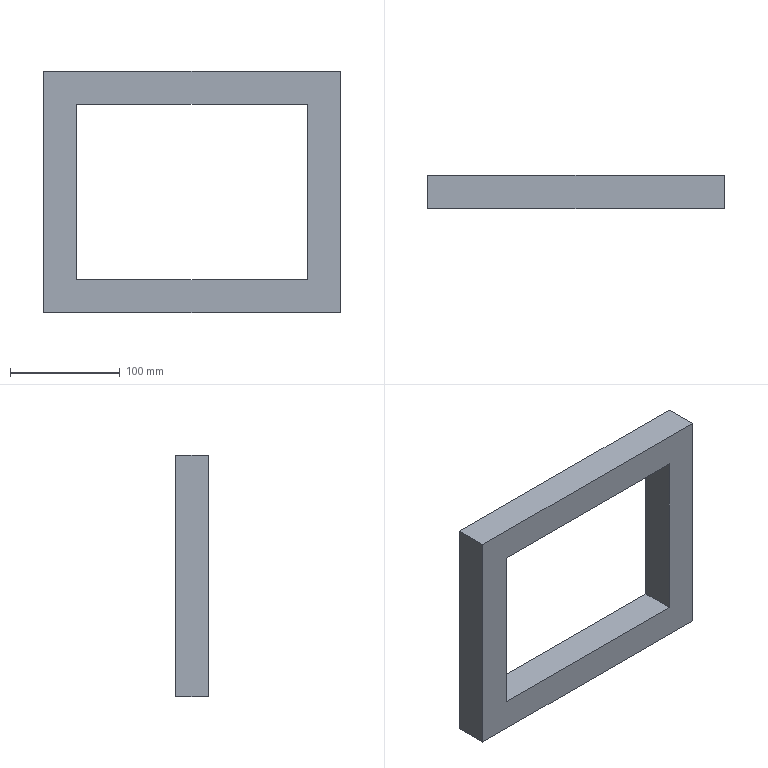Part | SolidWorks | features Extrusion 1, HoleWzd 1 | 1 solid | 58 faces | box 270 x 30 x 220 mm | volume 767460 mm3 | cone 32 | cylinder 16 | plane 10 | commonest cylinder face diameters 6.8 x16
STEP:
#1=CARTESIAN_POINT('',(0.,29.375,-98.4));
#2=VERTEX_POINT('',#1);
#3=CARTESIAN_POINT('',(0.,29.375,-91.6));
#4=VERTEX_POINT('',#3);
#5=CARTESIAN_POINT('',(0.,29.375,-95.));
#6=DIRECTION('',(0.,1.,0.));
#7=DIRECTION('',(0.,0.,1.));
#8=AXIS2_PLACEMENT_3D('',#5,#6,#7);
#9=CIRCLE('',#8,3.4);
#10=EDGE_CURVE('',#2,#4,#9,.T.);
#11=ORIENTED_EDGE('',*,*,#10,.F.);
#12=CARTESIAN_POINT('',(0.,30.,-99.025));
#13=VERTEX_POINT('',#12);
#14=CARTESIAN_POINT('',(0.,30.,-99.025));
#15=DIRECTION('',(0.,0.7071,-0.7071));
#16=VECTOR('',#15,1000.);
#17=LINE('',#14,#16);
#18=EDGE_CURVE('',#2,#13,#17,.T.);
#19=ORIENTED_EDGE('',*,*,#18,.T.);
#20=CARTESIAN_POINT('',(0.,30.,-90.975));
#21=VERTEX_POINT('',#20);
#22=CARTESIAN_POINT('',(0.,30.,-95.));
#23=DIRECTION('',(0.,1.,0.));
#24=DIRECTION('',(0.,0.,1.));
#25=AXIS2_PLACEMENT_3D('',#22,#23,#24);
#26=CIRCLE('',#25,4.025);
#27=EDGE_CURVE('',#13,#21,#26,.T.);
#28=ORIENTED_EDGE('',*,*,#27,.T.);
#29=CARTESIAN_POINT('',(0.,30.,-90.975));
#30=DIRECTION('',(0.,0.7071,0.7071));
#31=VECTOR('',#30,1000.);
#32=LINE('',#29,#31);
#33=EDGE_CURVE('',#4,#21,#32,.T.);
#34=ORIENTED_EDGE('',*,*,#33,.F.);
#35=EDGE_LOOP('',(#11,#19,#28,#34));
#36=FACE_OUTER_BOUND('',#35,.T.);
#37=CARTESIAN_POINT('',(0.,30.,-95.));
#38=DIRECTION('',(0.,1.,0.));
#39=DIRECTION('',(0.,0.,1.));
#40=AXIS2_PLACEMENT_3D('',#37,#38,#39);
#41=CONICAL_SURFACE('',#40,4.025,0.7854);
#42=ADVANCED_FACE('',(#36),#41,.F.);
#43=CARTESIAN_POINT('',(0.,8.293,-98.4));
#44=VERTEX_POINT('',#43);
#45=CARTESIAN_POINT('',(0.,8.293,-91.6));
#46=VERTEX_POINT('',#45);
#47=CARTESIAN_POINT('',(0.,8.293,-95.));
#48=DIRECTION('',(0.,1.,0.));
#49=DIRECTION('',(0.,0.,1.));
#50=AXIS2_PLACEMENT_3D('',#47,#48,#49);
#51=CIRCLE('',#50,3.4);
#52=EDGE_CURVE('',#44,#46,#51,.T.);
#53=ORIENTED_EDGE('',*,*,#52,.F.);
#54=CARTESIAN_POINT('',(0.,30.,-98.4));
#55=DIRECTION('',(0.,1.,0.));
#56=VECTOR('',#55,1000.);
#57=LINE('',#54,#56);
#58=EDGE_CURVE('',#44,#2,#57,.T.);
#59=ORIENTED_EDGE('',*,*,#58,.T.);
#60=ORIENTED_EDGE('',*,*,#10,.T.);
#61=CARTESIAN_POINT('',(0.,30.,-91.6));
#62=DIRECTION('',(0.,1.,0.));
#63=VECTOR('',#62,1000.);
#64=LINE('',#61,#63);
#65=EDGE_CURVE('',#46,#4,#64,.T.);
#66=ORIENTED_EDGE('',*,*,#65,.F.);
#67=EDGE_LOOP('',(#53,#59,#60,#66));
#68=FACE_OUTER_BOUND('',#67,.T.);
#69=CARTESIAN_POINT('',(0.,30.,-95.));
#70=DIRECTION('',(0.,1.,0.));
#71=DIRECTION('',(0.,0.,1.));
#72=AXIS2_PLACEMENT_3D('',#69,#70,#71);
#73=CYLINDRICAL_SURFACE('',#72,3.4);
#74=ADVANCED_FACE('',(#68),#73,.F.);
#75=CARTESIAN_POINT('',(0.,6.25,-95.));
#76=VERTEX_POINT('',#75);
#77=CARTESIAN_POINT('',(0.,8.293,-91.6));
#78=DIRECTION('',(0.,0.515,0.8572));
#79=VECTOR('',#78,1000.);
#80=LINE('',#77,#79);
#81=EDGE_CURVE('',#76,#46,#80,.T.);
#82=ORIENTED_EDGE('',*,*,#81,.F.);
#83=CARTESIAN_POINT('',(0.,8.293,-98.4));
#84=DIRECTION('',(0.,0.515,-0.8572));
#85=VECTOR('',#84,1000.);
#86=LINE('',#83,#85);
#87=EDGE_CURVE('',#76,#44,#86,.T.);
#88=ORIENTED_EDGE('',*,*,#87,.T.);
#89=ORIENTED_EDGE('',*,*,#52,.T.);
#90=EDGE_LOOP('',(#82,#88,#89));
#91=FACE_OUTER_BOUND('',#90,.T.);
#92=CARTESIAN_POINT('',(0.,8.293,-95.));
#93=DIRECTION('',(0.,1.,0.));
#94=DIRECTION('',(0.,0.,1.));
#95=AXIS2_PLACEMENT_3D('',#92,#93,#94);
#96=CONICAL_SURFACE('',#95,3.4,1.03);
#97=ADVANCED_FACE('',(#91),#96,.F.);
#98=CARTESIAN_POINT('',(-120.,29.375,-98.4));
#99=VERTEX_POINT('',#98);
#100=CARTESIAN_POINT('',(-120.,29.375,-91.6));
#101=VERTEX_POINT('',#100);
#102=CARTESIAN_POINT('',(-120.,29.375,-95.));
#103=DIRECTION('',(0.,1.,0.));
#104=DIRECTION('',(0.,0.,1.));
#105=AXIS2_PLACEMENT_3D('',#102,#103,#104);
#106=CIRCLE('',#105,3.4);
#107=EDGE_CURVE('',#99,#101,#106,.T.);
#108=ORIENTED_EDGE('',*,*,#107,.F.);
#109=CARTESIAN_POINT('',(-120.,30.,-99.025));
#110=VERTEX_POINT('',#109);
#111=CARTESIAN_POINT('',(-120.,30.,-99.025));
#112=DIRECTION('',(0.,0.7071,-0.7071));
#113=VECTOR('',#112,1000.);
#114=LINE('',#111,#113);
#115=EDGE_CURVE('',#99,#110,#114,.T.);
#116=ORIENTED_EDGE('',*,*,#115,.T.);
#117=CARTESIAN_POINT('',(-120.,30.,-90.975));
#118=VERTEX_POINT('',#117);
#119=CARTESIAN_POINT('',(-120.,30.,-95.));
#120=DIRECTION('',(0.,1.,0.));
#121=DIRECTION('',(0.,0.,1.));
#122=AXIS2_PLACEMENT_3D('',#119,#120,#121);
#123=CIRCLE('',#122,4.025);
#124=EDGE_CURVE('',#110,#118,#123,.T.);
#125=ORIENTED_EDGE('',*,*,#124,.T.);
#126=CARTESIAN_POINT('',(-120.,30.,-90.975));
#127=DIRECTION('',(0.,0.7071,0.7071));
#128=VECTOR('',#127,1000.);
#129=LINE('',#126,#128);
#130=EDGE_CURVE('',#101,#118,#129,.T.);
#131=ORIENTED_EDGE('',*,*,#130,.F.);
#132=EDGE_LOOP('',(#108,#116,#125,#131));
#133=FACE_OUTER_BOUND('',#132,.T.);
#134=CARTESIAN_POINT('',(-120.,30.,-95.));
#135=DIRECTION('',(0.,1.,0.));
#136=DIRECTION('',(0.,0.,1.));
#137=AXIS2_PLACEMENT_3D('',#134,#135,#136);
#138=CONICAL_SURFACE('',#137,4.025,0.7854);
#139=ADVANCED_FACE('',(#133),#138,.F.);
#140=CARTESIAN_POINT('',(-120.,8.293,-98.4));
#141=VERTEX_POINT('',#140);
#142=CARTESIAN_POINT('',(-120.,8.293,-91.6));
#143=VERTEX_POINT('',#142);
#144=CARTESIAN_POINT('',(-120.,8.293,-95.));
#145=DIRECTION('',(0.,1.,0.));
#146=DIRECTION('',(0.,0.,1.));
#147=AXIS2_PLACEMENT_3D('',#144,#145,#146);
#148=CIRCLE('',#147,3.4);
#149=EDGE_CURVE('',#141,#143,#148,.T.);
#150=ORIENTED_EDGE('',*,*,#149,.F.);
#151=CARTESIAN_POINT('',(-120.,30.,-98.4));
#152=DIRECTION('',(0.,1.,0.));
#153=VECTOR('',#152,1000.);
#154=LINE('',#151,#153);
#155=EDGE_CURVE('',#141,#99,#154,.T.);
#156=ORIENTED_EDGE('',*,*,#155,.T.);
#157=ORIENTED_EDGE('',*,*,#107,.T.);
#158=CARTESIAN_POINT('',(-120.,30.,-91.6));
#159=DIRECTION('',(0.,1.,0.));
#160=VECTOR('',#159,1000.);
#161=LINE('',#158,#160);
#162=EDGE_CURVE('',#143,#101,#161,.T.);
#163=ORIENTED_EDGE('',*,*,#162,.F.);
#164=EDGE_LOOP('',(#150,#156,#157,#163));
#165=FACE_OUTER_BOUND('',#164,.T.);
#166=CARTESIAN_POINT('',(-120.,30.,-95.));
#167=DIRECTION('',(0.,1.,0.));
#168=DIRECTION('',(0.,0.,1.));
#169=AXIS2_PLACEMENT_3D('',#166,#167,#168);
#170=CYLINDRICAL_SURFACE('',#169,3.4);
#171=ADVANCED_FACE('',(#165),#170,.F.);
#172=CARTESIAN_POINT('',(-120.,6.25,-95.));
#173=VERTEX_POINT('',#172);
#174=CARTESIAN_POINT('',(-120.,8.293,-91.6));
#175=DIRECTION('',(0.,0.515,0.8572));
#176=VECTOR('',#175,1000.);
#177=LINE('',#174,#176);
#178=EDGE_CURVE('',#173,#143,#177,.T.);
#179=ORIENTED_EDGE('',*,*,#178,.F.);
#180=CARTESIAN_POINT('',(-120.,8.293,-98.4));
#181=DIRECTION('',(0.,0.515,-0.8572));
#182=VECTOR('',#181,1000.);
#183=LINE('',#180,#182);
#184=EDGE_CURVE('',#173,#141,#183,.T.);
#185=ORIENTED_EDGE('',*,*,#184,.T.);
#186=ORIENTED_EDGE('',*,*,#149,.T.);
#187=EDGE_LOOP('',(#179,#185,#186));
#188=FACE_OUTER_BOUND('',#187,.T.);
#189=CARTESIAN_POINT('',(-120.,8.293,-95.));
#190=DIRECTION('',(0.,1.,0.));
#191=DIRECTION('',(0.,0.,1.));
#192=AXIS2_PLACEMENT_3D('',#189,#190,#191);
#193=CONICAL_SURFACE('',#192,3.4,1.03);
#194=ADVANCED_FACE('',(#188),#193,.F.);
#195=CARTESIAN_POINT('',(-120.,29.375,-3.4));
#196=VERTEX_POINT('',#195);
#197=CARTESIAN_POINT('',(-120.,29.375,3.4));
#198=VERTEX_POINT('',#197);
#199=CARTESIAN_POINT('',(-120.,29.375,0.));
#200=DIRECTION('',(0.,1.,0.));
#201=DIRECTION('',(0.,0.,1.));
#202=AXIS2_PLACEMENT_3D('',#199,#200,#201);
#203=CIRCLE('',#202,3.4);
#204=EDGE_CURVE('',#196,#198,#203,.T.);
#205=ORIENTED_EDGE('',*,*,#204,.F.);
#206=CARTESIAN_POINT('',(-120.,30.,-4.025));
#207=VERTEX_POINT('',#206);
#208=CARTESIAN_POINT('',(-120.,30.,-4.025));
#209=DIRECTION('',(0.,0.7071,-0.7071));
#210=VECTOR('',#209,1000.);
#211=LINE('',#208,#210);
#212=EDGE_CURVE('',#196,#207,#211,.T.);
#213=ORIENTED_EDGE('',*,*,#212,.T.);
#214=CARTESIAN_POINT('',(-120.,30.,4.025));
#215=VERTEX_POINT('',#214);
#216=CARTESIAN_POINT('',(-120.,30.,0.));
#217=DIRECTION('',(0.,1.,0.));
#218=DIRECTION('',(0.,0.,1.));
#219=AXIS2_PLACEMENT_3D('',#216,#217,#218);
#220=CIRCLE('',#219,4.025);
#221=EDGE_CURVE('',#207,#215,#220,.T.);
#222=ORIENTED_EDGE('',*,*,#221,.T.);
#223=CARTESIAN_POINT('',(-120.,30.,4.025));
#224=DIRECTION('',(0.,0.7071,0.7071));
#225=VECTOR('',#224,1000.);
#226=LINE('',#223,#225);
#227=EDGE_CURVE('',#198,#215,#226,.T.);
#228=ORIENTED_EDGE('',*,*,#227,.F.);
#229=EDGE_LOOP('',(#205,#213,#222,#228));
#230=FACE_OUTER_BOUND('',#229,.T.);
#231=CARTESIAN_POINT('',(-120.,30.,0.));
#232=DIRECTION('',(0.,1.,0.));
#233=DIRECTION('',(0.,0.,1.));
#234=AXIS2_PLACEMENT_3D('',#231,#232,#233);
#235=CONICAL_SURFACE('',#234,4.025,0.7854);
#236=ADVANCED_FACE('',(#230),#235,.F.);
#237=CARTESIAN_POINT('',(-120.,8.293,-3.4));
#238=VERTEX_POINT('',#237);
#239=CARTESIAN_POINT('',(-120.,8.293,3.4));
#240=VERTEX_POINT('',#239);
#241=CARTESIAN_POINT('',(-120.,8.293,0.));
#242=DIRECTION('',(0.,1.,0.));
#243=DIRECTION('',(0.,0.,1.));
#244=AXIS2_PLACEMENT_3D('',#241,#242,#243);
#245=CIRCLE('',#244,3.4);
#246=EDGE_CURVE('',#238,#240,#245,.T.);
#247=ORIENTED_EDGE('',*,*,#246,.F.);
#248=CARTESIAN_POINT('',(-120.,30.,-3.4));
#249=DIRECTION('',(0.,1.,0.));
#250=VECTOR('',#249,1000.);
#251=LINE('',#248,#250);
#252=EDGE_CURVE('',#238,#196,#251,.T.);
#253=ORIENTED_EDGE('',*,*,#252,.T.);
#254=ORIENTED_EDGE('',*,*,#204,.T.);
#255=CARTESIAN_POINT('',(-120.,30.,3.4));
#256=DIRECTION('',(0.,1.,0.));
#257=VECTOR('',#256,1000.);
#258=LINE('',#255,#257);
#259=EDGE_CURVE('',#240,#198,#258,.T.);
#260=ORIENTED_EDGE('',*,*,#259,.F.);
#261=EDGE_LOOP('',(#247,#253,#254,#260));
#262=FACE_OUTER_BOUND('',#261,.T.);
#263=CARTESIAN_POINT('',(-120.,30.,0.));
#264=DIRECTION('',(0.,1.,0.));
#265=DIRECTION('',(0.,0.,1.));
#266=AXIS2_PLACEMENT_3D('',#263,#264,#265);
#267=CYLINDRICAL_SURFACE('',#266,3.4);
#268=ADVANCED_FACE('',(#262),#267,.F.);
#269=CARTESIAN_POINT('',(-120.,6.25,0.));
#270=VERTEX_POINT('',#269);
#271=CARTESIAN_POINT('',(-120.,8.293,3.4));
#272=DIRECTION('',(0.,0.515,0.8572));
#273=VECTOR('',#272,1000.);
#274=LINE('',#271,#273);
#275=EDGE_CURVE('',#270,#240,#274,.T.);
#276=ORIENTED_EDGE('',*,*,#275,.F.);
#277=CARTESIAN_POINT('',(-120.,8.293,-3.4));
#278=DIRECTION('',(0.,0.515,-0.8572));
#279=VECTOR('',#278,1000.);
#280=LINE('',#277,#279);
#281=EDGE_CURVE('',#270,#238,#280,.T.);
#282=ORIENTED_EDGE('',*,*,#281,.T.);
#283=ORIENTED_EDGE('',*,*,#246,.T.);
#284=EDGE_LOOP('',(#276,#282,#283));
#285=FACE_OUTER_BOUND('',#284,.T.);
#286=CARTESIAN_POINT('',(-120.,8.293,0.));
#287=DIRECTION('',(0.,1.,0.));
#288=DIRECTION('',(0.,0.,1.));
#289=AXIS2_PLACEMENT_3D('',#286,#287,#288);
#290=CONICAL_SURFACE('',#289,3.4,1.03);
#291=ADVANCED_FACE('',(#285),#290,.F.);
#292=CARTESIAN_POINT('',(-120.,29.375,91.6));
#293=VERTEX_POINT('',#292);
#294=CARTESIAN_POINT('',(-120.,29.375,98.4));
#295=VERTEX_POINT('',#294);
#296=CARTESIAN_POINT('',(-120.,29.375,95.));
#297=DIRECTION('',(0.,1.,0.));
#298=DIRECTION('',(0.,0.,1.));
#299=AXIS2_PLACEMENT_3D('',#296,#297,#298);
#300=CIRCLE('',#299,3.4);
#301=EDGE_CURVE('',#293,#295,#300,.T.);
#302=ORIENTED_EDGE('',*,*,#301,.F.);
#303=CARTESIAN_POINT('',(-120.,30.,90.975));
#304=VERTEX_POINT('',#303);
#305=CARTESIAN_POINT('',(-120.,30.,90.975));
#306=DIRECTION('',(0.,0.7071,-0.7071));
#307=VECTOR('',#306,1000.);
#308=LINE('',#305,#307);
#309=EDGE_CURVE('',#293,#304,#308,.T.);
#310=ORIENTED_EDGE('',*,*,#309,.T.);
#311=CARTESIAN_POINT('',(-120.,30.,99.025));
#312=VERTEX_POINT('',#311);
#313=CARTESIAN_POINT('',(-120.,30.,95.));
#314=DIRECTION('',(0.,1.,0.));
#315=DIRECTION('',(0.,0.,1.));
#316=AXIS2_PLACEMENT_3D('',#313,#314,#315);
#317=CIRCLE('',#316,4.025);
#318=EDGE_CURVE('',#304,#312,#317,.T.);
#319=ORIENTED_EDGE('',*,*,#318,.T.);
#320=CARTESIAN_POINT('',(-120.,30.,99.025));
#321=DIRECTION('',(0.,0.7071,0.7071));
#322=VECTOR('',#321,1000.);
#323=LINE('',#320,#322);
#324=EDGE_CURVE('',#295,#312,#323,.T.);
#325=ORIENTED_EDGE('',*,*,#324,.F.);
#326=EDGE_LOOP('',(#302,#310,#319,#325));
#327=FACE_OUTER_BOUND('',#326,.T.);
#328=CARTESIAN_POINT('',(-120.,30.,95.));
#329=DIRECTION('',(0.,1.,0.));
#330=DIRECTION('',(0.,0.,1.));
#331=AXIS2_PLACEMENT_3D('',#328,#329,#330);
#332=CONICAL_SURFACE('',#331,4.025,0.7854);
#333=ADVANCED_FACE('',(#327),#332,.F.);
#334=CARTESIAN_POINT('',(-120.,8.293,91.6));
#335=VERTEX_POINT('',#334);
#336=CARTESIAN_POINT('',(-120.,8.293,98.4));
#337=VERTEX_POINT('',#336);
#338=CARTESIAN_POINT('',(-120.,8.293,95.));
#339=DIRECTION('',(0.,1.,0.));
#340=DIRECTION('',(0.,0.,1.));
#341=AXIS2_PLACEMENT_3D('',#338,#339,#340);
#342=CIRCLE('',#341,3.4);
#343=EDGE_CURVE('',#335,#337,#342,.T.);
#344=ORIENTED_EDGE('',*,*,#343,.F.);
#345=CARTESIAN_POINT('',(-120.,30.,91.6));
#346=DIRECTION('',(0.,1.,0.));
#347=VECTOR('',#346,1000.);
#348=LINE('',#345,#347);
#349=EDGE_CURVE('',#335,#293,#348,.T.);
#350=ORIENTED_EDGE('',*,*,#349,.T.);
#351=ORIENTED_EDGE('',*,*,#301,.T.);
#352=CARTESIAN_POINT('',(-120.,30.,98.4));
#353=DIRECTION('',(0.,1.,0.));
#354=VECTOR('',#353,1000.);
#355=LINE('',#352,#354);
#356=EDGE_CURVE('',#337,#295,#355,.T.);
#357=ORIENTED_EDGE('',*,*,#356,.F.);
#358=EDGE_LOOP('',(#344,#350,#351,#357));
#359=FACE_OUTER_BOUND('',#358,.T.);
#360=CARTESIAN_POINT('',(-120.,30.,95.));
#361=DIRECTION('',(0.,1.,0.));
#362=DIRECTION('',(0.,0.,1.));
#363=AXIS2_PLACEMENT_3D('',#360,#361,#362);
#364=CYLINDRICAL_SURFACE('',#363,3.4);
#365=ADVANCED_FACE('',(#359),#364,.F.);
#366=CARTESIAN_POINT('',(-120.,6.25,95.));
#367=VERTEX_POINT('',#366);
#368=CARTESIAN_POINT('',(-120.,8.293,98.4));
#369=DIRECTION('',(0.,0.515,0.8572));
#370=VECTOR('',#369,1000.);
#371=LINE('',#368,#370);
#372=EDGE_CURVE('',#367,#337,#371,.T.);
#373=ORIENTED_EDGE('',*,*,#372,.F.);
#374=CARTESIAN_POINT('',(-120.,8.293,91.6));
#375=DIRECTION('',(0.,0.515,-0.8572));
#376=VECTOR('',#375,1000.);
#377=LINE('',#374,#376);
#378=EDGE_CURVE('',#367,#335,#377,.T.);
#379=ORIENTED_EDGE('',*,*,#378,.T.);
#380=ORIENTED_EDGE('',*,*,#343,.T.);
#381=EDGE_LOOP('',(#373,#379,#380));
#382=FACE_OUTER_BOUND('',#381,.T.);
#383=CARTESIAN_POINT('',(-120.,8.293,95.));
#384=DIRECTION('',(0.,1.,0.));
#385=DIRECTION('',(0.,0.,1.));
#386=AXIS2_PLACEMENT_3D('',#383,#384,#385);
#387=CONICAL_SURFACE('',#386,3.4,1.03);
#388=ADVANCED_FACE('',(#382),#387,.F.);
#389=CARTESIAN_POINT('',(0.,29.375,91.6));
#390=VERTEX_POINT('',#389);
#391=CARTESIAN_POINT('',(0.,29.375,98.4));
#392=VERTEX_POINT('',#391);
#393=CARTESIAN_POINT('',(0.,29.375,95.));
#394=DIRECTION('',(0.,1.,0.));
#395=DIRECTION('',(0.,0.,1.));
#396=AXIS2_PLACEMENT_3D('',#393,#394,#395);
#397=CIRCLE('',#396,3.4);
#398=EDGE_CURVE('',#390,#392,#397,.T.);
#399=ORIENTED_EDGE('',*,*,#398,.F.);
#400=CARTESIAN_POINT('',(0.,30.,90.975));
#401=VERTEX_POINT('',#400);
#402=CARTESIAN_POINT('',(0.,30.,90.975));
#403=DIRECTION('',(0.,0.7071,-0.7071));
#404=VECTOR('',#403,1000.);
#405=LINE('',#402,#404);
#406=EDGE_CURVE('',#390,#401,#405,.T.);
#407=ORIENTED_EDGE('',*,*,#406,.T.);
#408=CARTESIAN_POINT('',(0.,30.,99.025));
#409=VERTEX_POINT('',#408);
#410=CARTESIAN_POINT('',(0.,30.,95.));
#411=DIRECTION('',(0.,1.,0.));
#412=DIRECTION('',(0.,0.,1.));
#413=AXIS2_PLACEMENT_3D('',#410,#411,#412);
#414=CIRCLE('',#413,4.025);
#415=EDGE_CURVE('',#401,#409,#414,.T.);
#416=ORIENTED_EDGE('',*,*,#415,.T.);
#417=CARTESIAN_POINT('',(0.,30.,99.025));
#418=DIRECTION('',(0.,0.7071,0.7071));
#419=VECTOR('',#418,1000.);
#420=LINE('',#417,#419);
#421=EDGE_CURVE('',#392,#409,#420,.T.);
#422=ORIENTED_EDGE('',*,*,#421,.F.);
#423=EDGE_LOOP('',(#399,#407,#416,#422));
#424=FACE_OUTER_BOUND('',#423,.T.);
#425=CARTESIAN_POINT('',(0.,30.,95.));
#426=DIRECTION('',(0.,1.,0.));
#427=DIRECTION('',(0.,0.,1.));
#428=AXIS2_PLACEMENT_3D('',#425,#426,#427);
#429=CONICAL_SURFACE('',#428,4.025,0.7854);
#430=ADVANCED_FACE('',(#424),#429,.F.);
#431=CARTESIAN_POINT('',(0.,8.293,91.6));
#432=VERTEX_POINT('',#431);
#433=CARTESIAN_POINT('',(0.,8.293,98.4));
#434=VERTEX_POINT('',#433);
#435=CARTESIAN_POINT('',(0.,8.293,95.));
#436=DIRECTION('',(0.,1.,0.));
#437=DIRECTION('',(0.,0.,1.));
#438=AXIS2_PLACEMENT_3D('',#435,#436,#437);
#439=CIRCLE('',#438,3.4);
#440=EDGE_CURVE('',#432,#434,#439,.T.);
#441=ORIENTED_EDGE('',*,*,#440,.F.);
#442=CARTESIAN_POINT('',(0.,30.,91.6));
#443=DIRECTION('',(0.,1.,0.));
#444=VECTOR('',#443,1000.);
#445=LINE('',#442,#444);
#446=EDGE_CURVE('',#432,#390,#445,.T.);
#447=ORIENTED_EDGE('',*,*,#446,.T.);
#448=ORIENTED_EDGE('',*,*,#398,.T.);
#449=CARTESIAN_POINT('',(0.,30.,98.4));
#450=DIRECTION('',(0.,1.,0.));
#451=VECTOR('',#450,1000.);
#452=LINE('',#449,#451);
#453=EDGE_CURVE('',#434,#392,#452,.T.);
#454=ORIENTED_EDGE('',*,*,#453,.F.);
#455=EDGE_LOOP('',(#441,#447,#448,#454));
#456=FACE_OUTER_BOUND('',#455,.T.);
#457=CARTESIAN_POINT('',(0.,30.,95.));
#458=DIRECTION('',(0.,1.,0.));
#459=DIRECTION('',(0.,0.,1.));
#460=AXIS2_PLACEMENT_3D('',#457,#458,#459);
#461=CYLINDRICAL_SURFACE('',#460,3.4);
#462=ADVANCED_FACE('',(#456),#461,.F.);
#463=CARTESIAN_POINT('',(0.,6.25,95.));
#464=VERTEX_POINT('',#463);
#465=CARTESIAN_POINT('',(0.,8.293,98.4));
#466=DIRECTION('',(0.,0.515,0.8572));
#467=VECTOR('',#466,1000.);
#468=LINE('',#465,#467);
#469=EDGE_CURVE('',#464,#434,#468,.T.);
#470=ORIENTED_EDGE('',*,*,#469,.F.);
#471=CARTESIAN_POINT('',(0.,8.293,91.6));
#472=DIRECTION('',(0.,0.515,-0.8572));
#473=VECTOR('',#472,1000.);
#474=LINE('',#471,#473);
#475=EDGE_CURVE('',#464,#432,#474,.T.);
#476=ORIENTED_EDGE('',*,*,#475,.T.);
#477=ORIENTED_EDGE('',*,*,#440,.T.);
#478=EDGE_LOOP('',(#470,#476,#477));
#479=FACE_OUTER_BOUND('',#478,.T.);
#480=CARTESIAN_POINT('',(0.,8.293,95.));
#481=DIRECTION('',(0.,1.,0.));
#482=DIRECTION('',(0.,0.,1.));
#483=AXIS2_PLACEMENT_3D('',#480,#481,#482);
#484=CONICAL_SURFACE('',#483,3.4,1.03);
#485=ADVANCED_FACE('',(#479),#484,.F.);
#486=CARTESIAN_POINT('',(120.,29.375,91.6));
#487=VERTEX_POINT('',#486);
#488=CARTESIAN_POINT('',(120.,29.375,98.4));
#489=VERTEX_POINT('',#488);
#490=CARTESIAN_POINT('',(120.,29.375,95.));
#491=DIRECTION('',(0.,1.,0.));
#492=DIRECTION('',(0.,0.,1.));
#493=AXIS2_PLACEMENT_3D('',#490,#491,#492);
#494=CIRCLE('',#493,3.4);
#495=EDGE_CURVE('',#487,#489,#494,.T.);
#496=ORIENTED_EDGE('',*,*,#495,.F.);
#497=CARTESIAN_POINT('',(120.,30.,90.975));
#498=VERTEX_POINT('',#497);
#499=CARTESIAN_POINT('',(120.,30.,90.975));
#500=DIRECTION('',(0.,0.7071,-0.7071));
#501=VECTOR('',#500,1000.);
#502=LINE('',#499,#501);
#503=EDGE_CURVE('',#487,#498,#502,.T.);
#504=ORIENTED_EDGE('',*,*,#503,.T.);
#505=CARTESIAN_POINT('',(120.,30.,99.025));
#506=VERTEX_POINT('',#505);
#507=CARTESIAN_POINT('',(120.,30.,95.));
#508=DIRECTION('',(0.,1.,0.));
#509=DIRECTION('',(0.,0.,1.));
#510=AXIS2_PLACEMENT_3D('',#507,#508,#509);
#511=CIRCLE('',#510,4.025);
#512=EDGE_CURVE('',#498,#506,#511,.T.);
#513=ORIENTED_EDGE('',*,*,#512,.T.);
#514=CARTESIAN_POINT('',(120.,30.,99.025));
#515=DIRECTION('',(0.,0.7071,0.7071));
#516=VECTOR('',#515,1000.);
#517=LINE('',#514,#516);
#518=EDGE_CURVE('',#489,#506,#517,.T.);
#519=ORIENTED_EDGE('',*,*,#518,.F.);
#520=EDGE_LOOP('',(#496,#504,#513,#519));
#521=FACE_OUTER_BOUND('',#520,.T.);
#522=CARTESIAN_POINT('',(120.,30.,95.));
#523=DIRECTION('',(0.,1.,0.));
#524=DIRECTION('',(0.,0.,1.));
#525=AXIS2_PLACEMENT_3D('',#522,#523,#524);
#526=CONICAL_SURFACE('',#525,4.025,0.7854);
#527=ADVANCED_FACE('',(#521),#526,.F.);
#528=CARTESIAN_POINT('',(120.,8.293,91.6));
#529=VERTEX_POINT('',#528);
#530=CARTESIAN_POINT('',(120.,8.293,98.4));
#531=VERTEX_POINT('',#530);
#532=CARTESIAN_POINT('',(120.,8.293,95.));
#533=DIRECTION('',(0.,1.,0.));
#534=DIRECTION('',(0.,0.,1.));
#535=AXIS2_PLACEMENT_3D('',#532,#533,#534);
#536=CIRCLE('',#535,3.4);
#537=EDGE_CURVE('',#529,#531,#536,.T.);
#538=ORIENTED_EDGE('',*,*,#537,.F.);
#539=CARTESIAN_POINT('',(120.,30.,91.6));
#540=DIRECTION('',(0.,1.,0.));
#541=VECTOR('',#540,1000.);
#542=LINE('',#539,#541);
#543=EDGE_CURVE('',#529,#487,#542,.T.);
#544=ORIENTED_EDGE('',*,*,#543,.T.);
#545=ORIENTED_EDGE('',*,*,#495,.T.);
#546=CARTESIAN_POINT('',(120.,30.,98.4));
#547=DIRECTION('',(0.,1.,0.));
#548=VECTOR('',#547,1000.);
#549=LINE('',#546,#548);
#550=EDGE_CURVE('',#531,#489,#549,.T.);
#551=ORIENTED_EDGE('',*,*,#550,.F.);
#552=EDGE_LOOP('',(#538,#544,#545,#551));
#553=FACE_OUTER_BOUND('',#552,.T.);
#554=CARTESIAN_POINT('',(120.,30.,95.));
#555=DIRECTION('',(0.,1.,0.));
#556=DIRECTION('',(0.,0.,1.));
#557=AXIS2_PLACEMENT_3D('',#554,#555,#556);
#558=CYLINDRICAL_SURFACE('',#557,3.4);
#559=ADVANCED_FACE('',(#553),#558,.F.);
#560=CARTESIAN_POINT('',(120.,6.25,95.));
#561=VERTEX_POINT('',#560);
#562=CARTESIAN_POINT('',(120.,8.293,98.4));
#563=DIRECTION('',(0.,0.515,0.8572));
#564=VECTOR('',#563,1000.);
#565=LINE('',#562,#564);
#566=EDGE_CURVE('',#561,#531,#565,.T.);
#567=ORIENTED_EDGE('',*,*,#566,.F.);
#568=CARTESIAN_POINT('',(120.,8.293,91.6));
#569=DIRECTION('',(0.,0.515,-0.8572));
#570=VECTOR('',#569,1000.);
#571=LINE('',#568,#570);
#572=EDGE_CURVE('',#561,#529,#571,.T.);
#573=ORIENTED_EDGE('',*,*,#572,.T.);
#574=ORIENTED_EDGE('',*,*,#537,.T.);
#575=EDGE_LOOP('',(#567,#573,#574));
#576=FACE_OUTER_BOUND('',#575,.T.);
#577=CARTESIAN_POINT('',(120.,8.293,95.));
#578=DIRECTION('',(0.,1.,0.));
#579=DIRECTION('',(0.,0.,1.));
#580=AXIS2_PLACEMENT_3D('',#577,#578,#579);
#581=CONICAL_SURFACE('',#580,3.4,1.03);
#582=ADVANCED_FACE('',(#576),#581,.F.);
#583=CARTESIAN_POINT('',(120.,29.375,-98.4));
#584=VERTEX_POINT('',#583);
#585=CARTESIAN_POINT('',(120.,29.375,-91.6));
#586=VERTEX_POINT('',#585);
#587=CARTESIAN_POINT('',(120.,29.375,-95.));
#588=DIRECTION('',(0.,1.,0.));
#589=DIRECTION('',(0.,0.,1.));
#590=AXIS2_PLACEMENT_3D('',#587,#588,#589);
#591=CIRCLE('',#590,3.4);
#592=EDGE_CURVE('',#584,#586,#591,.T.);
#593=ORIENTED_EDGE('',*,*,#592,.F.);
#594=CARTESIAN_POINT('',(120.,30.,-99.025));
#595=VERTEX_POINT('',#594);
#596=CARTESIAN_POINT('',(120.,30.,-99.025));
#597=DIRECTION('',(0.,0.7071,-0.7071));
#598=VECTOR('',#597,1000.);
#599=LINE('',#596,#598);
#600=EDGE_CURVE('',#584,#595,#599,.T.);
#601=ORIENTED_EDGE('',*,*,#600,.T.);
#602=CARTESIAN_POINT('',(120.,30.,-90.975));
#603=VERTEX_POINT('',#602);
#604=CARTESIAN_POINT('',(120.,30.,-95.));
#605=DIRECTION('',(0.,1.,0.));
#606=DIRECTION('',(0.,0.,1.));
#607=AXIS2_PLACEMENT_3D('',#604,#605,#606);
#608=CIRCLE('',#607,4.025);
#609=EDGE_CURVE('',#595,#603,#608,.T.);
#610=ORIENTED_EDGE('',*,*,#609,.T.);
#611=CARTESIAN_POINT('',(120.,30.,-90.975));
#612=DIRECTION('',(0.,0.7071,0.7071));
#613=VECTOR('',#612,1000.);
#614=LINE('',#611,#613);
#615=EDGE_CURVE('',#586,#603,#614,.T.);
#616=ORIENTED_EDGE('',*,*,#615,.F.);
#617=EDGE_LOOP('',(#593,#601,#610,#616));
#618=FACE_OUTER_BOUND('',#617,.T.);
#619=CARTESIAN_POINT('',(120.,30.,-95.));
#620=DIRECTION('',(0.,1.,0.));
#621=DIRECTION('',(0.,0.,1.));
#622=AXIS2_PLACEMENT_3D('',#619,#620,#621);
#623=CONICAL_SURFACE('',#622,4.025,0.7854);
#624=ADVANCED_FACE('',(#618),#623,.F.);
#625=CARTESIAN_POINT('',(120.,8.293,-98.4));
#626=VERTEX_POINT('',#625);
#627=CARTESIAN_POINT('',(120.,8.293,-91.6));
#628=VERTEX_POINT('',#627);
#629=CARTESIAN_POINT('',(120.,8.293,-95.));
#630=DIRECTION('',(0.,1.,0.));
#631=DIRECTION('',(0.,0.,1.));
#632=AXIS2_PLACEMENT_3D('',#629,#630,#631);
#633=CIRCLE('',#632,3.4);
#634=EDGE_CURVE('',#626,#628,#633,.T.);
#635=ORIENTED_EDGE('',*,*,#634,.F.);
#636=CARTESIAN_POINT('',(120.,30.,-98.4));
#637=DIRECTION('',(0.,1.,0.));
#638=VECTOR('',#637,1000.);
#639=LINE('',#636,#638);
#640=EDGE_CURVE('',#626,#584,#639,.T.);
#641=ORIENTED_EDGE('',*,*,#640,.T.);
#642=ORIENTED_EDGE('',*,*,#592,.T.);
#643=CARTESIAN_POINT('',(120.,30.,-91.6));
#644=DIRECTION('',(0.,1.,0.));
#645=VECTOR('',#644,1000.);
#646=LINE('',#643,#645);
#647=EDGE_CURVE('',#628,#586,#646,.T.);
#648=ORIENTED_EDGE('',*,*,#647,.F.);
#649=EDGE_LOOP('',(#635,#641,#642,#648));
#650=FACE_OUTER_BOUND('',#649,.T.);
#651=CARTESIAN_POINT('',(120.,30.,-95.));
#652=DIRECTION('',(0.,1.,0.));
#653=DIRECTION('',(0.,0.,1.));
#654=AXIS2_PLACEMENT_3D('',#651,#652,#653);
#655=CYLINDRICAL_SURFACE('',#654,3.4);
#656=ADVANCED_FACE('',(#650),#655,.F.);
#657=CARTESIAN_POINT('',(120.,6.25,-95.));
#658=VERTEX_POINT('',#657);
#659=CARTESIAN_POINT('',(120.,8.293,-91.6));
#660=DIRECTION('',(0.,0.515,0.8572));
#661=VECTOR('',#660,1000.);
#662=LINE('',#659,#661);
#663=EDGE_CURVE('',#658,#628,#662,.T.);
#664=ORIENTED_EDGE('',*,*,#663,.F.);
#665=CARTESIAN_POINT('',(120.,8.293,-98.4));
#666=DIRECTION('',(0.,0.515,-0.8572));
#667=VECTOR('',#666,1000.);
#668=LINE('',#665,#667);
#669=EDGE_CURVE('',#658,#626,#668,.T.);
#670=ORIENTED_EDGE('',*,*,#669,.T.);
#671=ORIENTED_EDGE('',*,*,#634,.T.);
#672=EDGE_LOOP('',(#664,#670,#671));
#673=FACE_OUTER_BOUND('',#672,.T.);
#674=CARTESIAN_POINT('',(120.,8.293,-95.));
#675=DIRECTION('',(0.,1.,0.));
#676=DIRECTION('',(0.,0.,1.));
#677=AXIS2_PLACEMENT_3D('',#674,#675,#676);
#678=CONICAL_SURFACE('',#677,3.4,1.03);
#679=ADVANCED_FACE('',(#673),#678,.F.);
#680=CARTESIAN_POINT('',(120.,29.375,-3.4));
#681=VERTEX_POINT('',#680);
#682=CARTESIAN_POINT('',(120.,29.375,3.4));
#683=VERTEX_POINT('',#682);
#684=CARTESIAN_POINT('',(120.,29.375,0.));
#685=DIRECTION('',(0.,1.,0.));
#686=DIRECTION('',(0.,0.,1.));
#687=AXIS2_PLACEMENT_3D('',#684,#685,#686);
#688=CIRCLE('',#687,3.4);
#689=EDGE_CURVE('',#681,#683,#688,.T.);
#690=ORIENTED_EDGE('',*,*,#689,.F.);
#691=CARTESIAN_POINT('',(120.,30.,-4.025));
#692=VERTEX_POINT('',#691);
#693=CARTESIAN_POINT('',(120.,30.,-4.025));
#694=DIRECTION('',(0.,0.7071,-0.7071));
#695=VECTOR('',#694,1000.);
#696=LINE('',#693,#695);
#697=EDGE_CURVE('',#681,#692,#696,.T.);
#698=ORIENTED_EDGE('',*,*,#697,.T.);
#699=CARTESIAN_POINT('',(120.,30.,4.025));
#700=VERTEX_POINT('',#699);
#701=CARTESIAN_POINT('',(120.,30.,0.));
#702=DIRECTION('',(0.,1.,0.));
#703=DIRECTION('',(0.,0.,1.));
#704=AXIS2_PLACEMENT_3D('',#701,#702,#703);
#705=CIRCLE('',#704,4.025);
#706=EDGE_CURVE('',#692,#700,#705,.T.);
#707=ORIENTED_EDGE('',*,*,#706,.T.);
#708=CARTESIAN_POINT('',(120.,30.,4.025));
#709=DIRECTION('',(0.,0.7071,0.7071));
#710=VECTOR('',#709,1000.);
#711=LINE('',#708,#710);
#712=EDGE_CURVE('',#683,#700,#711,.T.);
#713=ORIENTED_EDGE('',*,*,#712,.F.);
#714=EDGE_LOOP('',(#690,#698,#707,#713));
#715=FACE_OUTER_BOUND('',#714,.T.);
#716=CARTESIAN_POINT('',(120.,30.,0.));
#717=DIRECTION('',(0.,1.,0.));
#718=DIRECTION('',(0.,0.,1.));
#719=AXIS2_PLACEMENT_3D('',#716,#717,#718);
#720=CONICAL_SURFACE('',#719,4.025,0.7854);
#721=ADVANCED_FACE('',(#715),#720,.F.);
#722=CARTESIAN_POINT('',(120.,8.293,-3.4));
#723=VERTEX_POINT('',#722);
#724=CARTESIAN_POINT('',(120.,8.293,3.4));
#725=VERTEX_POINT('',#724);
#726=CARTESIAN_POINT('',(120.,8.293,0.));
#727=DIRECTION('',(0.,1.,0.));
#728=DIRECTION('',(0.,0.,1.));
#729=AXIS2_PLACEMENT_3D('',#726,#727,#728);
#730=CIRCLE('',#729,3.4);
#731=EDGE_CURVE('',#723,#725,#730,.T.);
#732=ORIENTED_EDGE('',*,*,#731,.F.);
#733=CARTESIAN_POINT('',(120.,30.,-3.4));
#734=DIRECTION('',(0.,1.,0.));
#735=VECTOR('',#734,1000.);
#736=LINE('',#733,#735);
#737=EDGE_CURVE('',#723,#681,#736,.T.);
#738=ORIENTED_EDGE('',*,*,#737,.T.);
#739=ORIENTED_EDGE('',*,*,#689,.T.);
#740=CARTESIAN_POINT('',(120.,30.,3.4));
#741=DIRECTION('',(0.,1.,0.));
#742=VECTOR('',#741,1000.);
#743=LINE('',#740,#742);
#744=EDGE_CURVE('',#725,#683,#743,.T.);
#745=ORIENTED_EDGE('',*,*,#744,.F.);
#746=EDGE_LOOP('',(#732,#738,#739,#745));
#747=FACE_OUTER_BOUND('',#746,.T.);
#748=CARTESIAN_POINT('',(120.,30.,0.));
#749=DIRECTION('',(0.,1.,0.));
#750=DIRECTION('',(0.,0.,1.));
#751=AXIS2_PLACEMENT_3D('',#748,#749,#750);
#752=CYLINDRICAL_SURFACE('',#751,3.4);
#753=ADVANCED_FACE('',(#747),#752,.F.);
#754=CARTESIAN_POINT('',(120.,6.25,0.));
#755=VERTEX_POINT('',#754);
#756=CARTESIAN_POINT('',(120.,8.293,3.4));
#757=DIRECTION('',(0.,0.515,0.8572));
#758=VECTOR('',#757,1000.);
#759=LINE('',#756,#758);
#760=EDGE_CURVE('',#755,#725,#759,.T.);
#761=ORIENTED_EDGE('',*,*,#760,.F.);
#762=CARTESIAN_POINT('',(120.,8.293,-3.4));
#763=DIRECTION('',(0.,0.515,-0.8572));
#764=VECTOR('',#763,1000.);
#765=LINE('',#762,#764);
#766=EDGE_CURVE('',#755,#723,#765,.T.);
#767=ORIENTED_EDGE('',*,*,#766,.T.);
#768=ORIENTED_EDGE('',*,*,#731,.T.);
#769=EDGE_LOOP('',(#761,#767,#768));
#770=FACE_OUTER_BOUND('',#769,.T.);
#771=CARTESIAN_POINT('',(120.,8.293,0.));
#772=DIRECTION('',(0.,1.,0.));
#773=DIRECTION('',(0.,0.,1.));
#774=AXIS2_PLACEMENT_3D('',#771,#772,#773);
#775=CONICAL_SURFACE('',#774,3.4,1.03);
#776=ADVANCED_FACE('',(#770),#775,.F.);
#777=CARTESIAN_POINT('',(0.,30.,-95.));
#778=DIRECTION('',(0.,1.,0.));
#779=DIRECTION('',(0.,0.,1.));
#780=AXIS2_PLACEMENT_3D('',#777,#778,#779);
#781=CIRCLE('',#780,4.025);
#782=EDGE_CURVE('',#21,#13,#781,.T.);
#783=ORIENTED_EDGE('',*,*,#782,.F.);
#784=ORIENTED_EDGE('',*,*,#27,.F.);
#785=EDGE_LOOP('',(#783,#784));
#786=FACE_BOUND('',#785,.T.);
#787=CARTESIAN_POINT('',(-120.,30.,-95.));
#788=DIRECTION('',(0.,1.,0.));
#789=DIRECTION('',(0.,0.,1.));
#790=AXIS2_PLACEMENT_3D('',#787,#788,#789);
#791=CIRCLE('',#790,4.025);
#792=EDGE_CURVE('',#118,#110,#791,.T.);
#793=ORIENTED_EDGE('',*,*,#792,.F.);
#794=ORIENTED_EDGE('',*,*,#124,.F.);
#795=EDGE_LOOP('',(#793,#794));
#796=FACE_BOUND('',#795,.T.);
#797=CARTESIAN_POINT('',(-120.,30.,0.));
#798=DIRECTION('',(0.,1.,0.));
#799=DIRECTION('',(0.,0.,1.));
#800=AXIS2_PLACEMENT_3D('',#797,#798,#799);
#801=CIRCLE('',#800,4.025);
#802=EDGE_CURVE('',#215,#207,#801,.T.);
#803=ORIENTED_EDGE('',*,*,#802,.F.);
#804=ORIENTED_EDGE('',*,*,#221,.F.);
#805=EDGE_LOOP('',(#803,#804));
#806=FACE_BOUND('',#805,.T.);
#807=CARTESIAN_POINT('',(-120.,30.,95.));
#808=DIRECTION('',(0.,1.,0.));
#809=DIRECTION('',(0.,0.,1.));
#810=AXIS2_PLACEMENT_3D('',#807,#808,#809);
#811=CIRCLE('',#810,4.025);
#812=EDGE_CURVE('',#312,#304,#811,.T.);
#813=ORIENTED_EDGE('',*,*,#812,.F.);
#814=ORIENTED_EDGE('',*,*,#318,.F.);
#815=EDGE_LOOP('',(#813,#814));
#816=FACE_BOUND('',#815,.T.);
#817=CARTESIAN_POINT('',(0.,30.,95.));
#818=DIRECTION('',(0.,1.,0.));
#819=DIRECTION('',(0.,0.,1.));
#820=AXIS2_PLACEMENT_3D('',#817,#818,#819);
#821=CIRCLE('',#820,4.025);
#822=EDGE_CURVE('',#409,#401,#821,.T.);
#823=ORIENTED_EDGE('',*,*,#822,.F.);
#824=ORIENTED_EDGE('',*,*,#415,.F.);
#825=EDGE_LOOP('',(#823,#824));
#826=FACE_BOUND('',#825,.T.);
#827=CARTESIAN_POINT('',(120.,30.,95.));
#828=DIRECTION('',(0.,1.,0.));
#829=DIRECTION('',(0.,0.,1.));
#830=AXIS2_PLACEMENT_3D('',#827,#828,#829);
#831=CIRCLE('',#830,4.025);
#832=EDGE_CURVE('',#506,#498,#831,.T.);
#833=ORIENTED_EDGE('',*,*,#832,.F.);
#834=ORIENTED_EDGE('',*,*,#512,.F.);
#835=EDGE_LOOP('',(#833,#834));
#836=FACE_BOUND('',#835,.T.);
#837=CARTESIAN_POINT('',(120.,30.,-95.));
#838=DIRECTION('',(0.,1.,0.));
#839=DIRECTION('',(0.,0.,1.));
#840=AXIS2_PLACEMENT_3D('',#837,#838,#839);
#841=CIRCLE('',#840,4.025);
#842=EDGE_CURVE('',#603,#595,#841,.T.);
#843=ORIENTED_EDGE('',*,*,#842,.F.);
#844=ORIENTED_EDGE('',*,*,#609,.F.);
#845=EDGE_LOOP('',(#843,#844));
#846=FACE_BOUND('',#845,.T.);
#847=CARTESIAN_POINT('',(120.,30.,0.));
#848=DIRECTION('',(0.,1.,0.));
#849=DIRECTION('',(0.,0.,1.));
#850=AXIS2_PLACEMENT_3D('',#847,#848,#849);
#851=CIRCLE('',#850,4.025);
#852=EDGE_CURVE('',#700,#692,#851,.T.);
#853=ORIENTED_EDGE('',*,*,#852,.F.);
#854=ORIENTED_EDGE('',*,*,#706,.F.);
#855=EDGE_LOOP('',(#853,#854));
#856=FACE_BOUND('',#855,.T.);
#857=CARTESIAN_POINT('',(135.,30.,110.));
#858=VERTEX_POINT('',#857);
#859=CARTESIAN_POINT('',(135.,30.,-110.));
#860=VERTEX_POINT('',#859);
#861=CARTESIAN_POINT('',(135.,30.,-110.));
#862=DIRECTION('',(0.,0.,-1.));
#863=VECTOR('',#862,1000.);
#864=LINE('',#861,#863);
#865=EDGE_CURVE('',#858,#860,#864,.T.);
#866=ORIENTED_EDGE('',*,*,#865,.T.);
#867=CARTESIAN_POINT('',(-135.,30.,-110.));
#868=VERTEX_POINT('',#867);
#869=CARTESIAN_POINT('',(-135.,30.,-110.));
#870=DIRECTION('',(-1.,0.,0.));
#871=VECTOR('',#870,1000.);
#872=LINE('',#869,#871);
#873=EDGE_CURVE('',#860,#868,#872,.T.);
#874=ORIENTED_EDGE('',*,*,#873,.T.);
#875=CARTESIAN_POINT('',(-135.,30.,110.));
#876=VERTEX_POINT('',#875);
#877=CARTESIAN_POINT('',(-135.,30.,-110.));
#878=DIRECTION('',(0.,0.,1.));
#879=VECTOR('',#878,1000.);
#880=LINE('',#877,#879);
#881=EDGE_CURVE('',#868,#876,#880,.T.);
#882=ORIENTED_EDGE('',*,*,#881,.T.);
#883=CARTESIAN_POINT('',(-135.,30.,110.));
#884=DIRECTION('',(1.,0.,0.));
#885=VECTOR('',#884,1000.);
#886=LINE('',#883,#885);
#887=EDGE_CURVE('',#876,#858,#886,.T.);
#888=ORIENTED_EDGE('',*,*,#887,.T.);
#889=EDGE_LOOP('',(#866,#874,#882,#888));
#890=FACE_OUTER_BOUND('',#889,.T.);
#891=CARTESIAN_POINT('',(105.,30.,-80.));
#892=VERTEX_POINT('',#891);
#893=CARTESIAN_POINT('',(-105.,30.,-80.));
#894=VERTEX_POINT('',#893);
#895=CARTESIAN_POINT('',(-105.,30.,-80.));
#896=DIRECTION('',(-1.,0.,0.));
#897=VECTOR('',#896,1000.);
#898=LINE('',#895,#897);
#899=EDGE_CURVE('',#892,#894,#898,.T.);
#900=ORIENTED_EDGE('',*,*,#899,.F.);
#901=CARTESIAN_POINT('',(105.,30.,80.));
#902=VERTEX_POINT('',#901);
#903=CARTESIAN_POINT('',(105.,30.,-80.));
#904=DIRECTION('',(0.,0.,-1.));
#905=VECTOR('',#904,1000.);
#906=LINE('',#903,#905);
#907=EDGE_CURVE('',#902,#892,#906,.T.);
#908=ORIENTED_EDGE('',*,*,#907,.F.);
#909=CARTESIAN_POINT('',(-105.,30.,80.));
#910=VERTEX_POINT('',#909);
#911=CARTESIAN_POINT('',(-105.,30.,80.));
#912=DIRECTION('',(1.,0.,0.));
#913=VECTOR('',#912,1000.);
#914=LINE('',#911,#913);
#915=EDGE_CURVE('',#910,#902,#914,.T.);
#916=ORIENTED_EDGE('',*,*,#915,.F.);
#917=CARTESIAN_POINT('',(-105.,30.,-80.));
#918=DIRECTION('',(0.,0.,1.));
#919=VECTOR('',#918,1000.);
#920=LINE('',#917,#919);
#921=EDGE_CURVE('',#894,#910,#920,.T.);
#922=ORIENTED_EDGE('',*,*,#921,.F.);
#923=EDGE_LOOP('',(#900,#908,#916,#922));
#924=FACE_BOUND('',#923,.T.);
#925=CARTESIAN_POINT('',(0.,30.,0.));
#926=DIRECTION('',(0.,1.,0.));
#927=DIRECTION('',(0.,0.,1.));
#928=AXIS2_PLACEMENT_3D('',#925,#926,#927);
#929=PLANE('',#928);
#930=ADVANCED_FACE('',(#786,#796,#806,#816,#826,#836,#846,#856,#890,#924),#929,.T.);
#931=CARTESIAN_POINT('',(135.,0.,110.));
#932=VERTEX_POINT('',#931);
#933=CARTESIAN_POINT('',(135.,0.,-110.));
#934=VERTEX_POINT('',#933);
#935=CARTESIAN_POINT('',(135.,0.,-110.));
#936=DIRECTION('',(0.,0.,-1.));
#937=VECTOR('',#936,1000.);
#938=LINE('',#935,#937);
#939=EDGE_CURVE('',#932,#934,#938,.T.);
#940=ORIENTED_EDGE('',*,*,#939,.F.);
#941=CARTESIAN_POINT('',(-135.,0.,110.));
#942=VERTEX_POINT('',#941);
#943=CARTESIAN_POINT('',(-135.,0.,110.));
#944=DIRECTION('',(1.,0.,0.));
#945=VECTOR('',#944,1000.);
#946=LINE('',#943,#945);
#947=EDGE_CURVE('',#942,#932,#946,.T.);
#948=ORIENTED_EDGE('',*,*,#947,.F.);
#949=CARTESIAN_POINT('',(-135.,0.,-110.));
#950=VERTEX_POINT('',#949);
#951=CARTESIAN_POINT('',(-135.,0.,-110.));
#952=DIRECTION('',(0.,0.,1.));
#953=VECTOR('',#952,1000.);
#954=LINE('',#951,#953);
#955=EDGE_CURVE('',#950,#942,#954,.T.);
#956=ORIENTED_EDGE('',*,*,#955,.F.);
#957=CARTESIAN_POINT('',(-135.,0.,-110.));
#958=DIRECTION('',(-1.,0.,0.));
#959=VECTOR('',#958,1000.);
#960=LINE('',#957,#959);
#961=EDGE_CURVE('',#934,#950,#960,.T.);
#962=ORIENTED_EDGE('',*,*,#961,.F.);
#963=EDGE_LOOP('',(#940,#948,#956,#962));
#964=FACE_OUTER_BOUND('',#963,.T.);
#965=CARTESIAN_POINT('',(105.,0.,80.));
#966=VERTEX_POINT('',#965);
#967=CARTESIAN_POINT('',(105.,0.,-80.));
#968=VERTEX_POINT('',#967);
#969=CARTESIAN_POINT('',(105.,0.,-80.));
#970=DIRECTION('',(0.,0.,-1.));
#971=VECTOR('',#970,1000.);
#972=LINE('',#969,#971);
#973=EDGE_CURVE('',#966,#968,#972,.T.);
#974=ORIENTED_EDGE('',*,*,#973,.T.);
#975=CARTESIAN_POINT('',(-105.,0.,-80.));
#976=VERTEX_POINT('',#975);
#977=CARTESIAN_POINT('',(-105.,0.,-80.));
#978=DIRECTION('',(-1.,0.,0.));
#979=VECTOR('',#978,1000.);
#980=LINE('',#977,#979);
#981=EDGE_CURVE('',#968,#976,#980,.T.);
#982=ORIENTED_EDGE('',*,*,#981,.T.);
#983=CARTESIAN_POINT('',(-105.,0.,80.));
#984=VERTEX_POINT('',#983);
#985=CARTESIAN_POINT('',(-105.,0.,-80.));
#986=DIRECTION('',(0.,0.,1.));
#987=VECTOR('',#986,1000.);
#988=LINE('',#985,#987);
#989=EDGE_CURVE('',#976,#984,#988,.T.);
#990=ORIENTED_EDGE('',*,*,#989,.T.);
#991=CARTESIAN_POINT('',(-105.,0.,80.));
#992=DIRECTION('',(1.,0.,0.));
#993=VECTOR('',#992,1000.);
#994=LINE('',#991,#993);
#995=EDGE_CURVE('',#984,#966,#994,.T.);
#996=ORIENTED_EDGE('',*,*,#995,.T.);
#997=EDGE_LOOP('',(#974,#982,#990,#996));
#998=FACE_BOUND('',#997,.T.);
#999=CARTESIAN_POINT('',(0.,0.,0.));
#1000=DIRECTION('',(0.,1.,0.));
#1001=DIRECTION('',(0.,0.,1.));
#1002=AXIS2_PLACEMENT_3D('',#999,#1000,#1001);
#1003=PLANE('',#1002);
#1004=ADVANCED_FACE('',(#964,#998),#1003,.F.);
#1005=ORIENTED_EDGE('',*,*,#939,.T.);
#1006=CARTESIAN_POINT('',(135.,30.,-110.));
#1007=DIRECTION('',(0.,-1.,0.));
#1008=VECTOR('',#1007,1000.);
#1009=LINE('',#1006,#1008);
#1010=EDGE_CURVE('',#860,#934,#1009,.T.);
#1011=ORIENTED_EDGE('',*,*,#1010,.F.);
#1012=ORIENTED_EDGE('',*,*,#865,.F.);
#1013=CARTESIAN_POINT('',(135.,30.,110.));
#1014=DIRECTION('',(0.,-1.,0.));
#1015=VECTOR('',#1014,1000.);
#1016=LINE('',#1013,#1015);
#1017=EDGE_CURVE('',#858,#932,#1016,.T.);
#1018=ORIENTED_EDGE('',*,*,#1017,.T.);
#1019=EDGE_LOOP('',(#1005,#1011,#1012,#1018));
#1020=FACE_OUTER_BOUND('',#1019,.T.);
#1021=CARTESIAN_POINT('',(135.,30.,-110.));
#1022=DIRECTION('',(-1.,0.,0.));
#1023=DIRECTION('',(0.,0.,1.));
#1024=AXIS2_PLACEMENT_3D('',#1021,#1022,#1023);
#1025=PLANE('',#1024);
#1026=ADVANCED_FACE('',(#1020),#1025,.F.);
#1027=ORIENTED_EDGE('',*,*,#961,.T.);
#1028=CARTESIAN_POINT('',(-135.,30.,-110.));
#1029=DIRECTION('',(0.,-1.,0.));
#1030=VECTOR('',#1029,1000.);
#1031=LINE('',#1028,#1030);
#1032=EDGE_CURVE('',#868,#950,#1031,.T.);
#1033=ORIENTED_EDGE('',*,*,#1032,.F.);
#1034=ORIENTED_EDGE('',*,*,#873,.F.);
#1035=ORIENTED_EDGE('',*,*,#1010,.T.);
#1036=EDGE_LOOP('',(#1027,#1033,#1034,#1035));
#1037=FACE_OUTER_BOUND('',#1036,.T.);
#1038=CARTESIAN_POINT('',(-135.,30.,-110.));
#1039=DIRECTION('',(0.,0.,1.));
#1040=DIRECTION('',(1.,0.,0.));
#1041=AXIS2_PLACEMENT_3D('',#1038,#1039,#1040);
#1042=PLANE('',#1041);
#1043=ADVANCED_FACE('',(#1037),#1042,.F.);
#1044=ORIENTED_EDGE('',*,*,#955,.T.);
#1045=CARTESIAN_POINT('',(-135.,30.,110.));
#1046=DIRECTION('',(0.,-1.,0.));
#1047=VECTOR('',#1046,1000.);
#1048=LINE('',#1045,#1047);
#1049=EDGE_CURVE('',#876,#942,#1048,.T.);
#1050=ORIENTED_EDGE('',*,*,#1049,.F.);
#1051=ORIENTED_EDGE('',*,*,#881,.F.);
#1052=ORIENTED_EDGE('',*,*,#1032,.T.);
#1053=EDGE_LOOP('',(#1044,#1050,#1051,#1052));
#1054=FACE_OUTER_BOUND('',#1053,.T.);
#1055=CARTESIAN_POINT('',(-135.,30.,-110.));
#1056=DIRECTION('',(1.,0.,0.));
#1057=DIRECTION('',(0.,0.,-1.));
#1058=AXIS2_PLACEMENT_3D('',#1055,#1056,#1057);
#1059=PLANE('',#1058);
#1060=ADVANCED_FACE('',(#1054),#1059,.F.);
#1061=ORIENTED_EDGE('',*,*,#947,.T.);
#1062=ORIENTED_EDGE('',*,*,#1017,.F.);
#1063=ORIENTED_EDGE('',*,*,#887,.F.);
#1064=ORIENTED_EDGE('',*,*,#1049,.T.);
#1065=EDGE_LOOP('',(#1061,#1062,#1063,#1064));
#1066=FACE_OUTER_BOUND('',#1065,.T.);
#1067=CARTESIAN_POINT('',(-135.,30.,110.));
#1068=DIRECTION('',(0.,0.,-1.));
#1069=DIRECTION('',(-1.,0.,0.));
#1070=AXIS2_PLACEMENT_3D('',#1067,#1068,#1069);
#1071=PLANE('',#1070);
#1072=ADVANCED_FACE('',(#1066),#1071,.F.);
#1073=ORIENTED_EDGE('',*,*,#973,.F.);
#1074=CARTESIAN_POINT('',(105.,30.,80.));
#1075=DIRECTION('',(0.,-1.,0.));
#1076=VECTOR('',#1075,1000.);
#1077=LINE('',#1074,#1076);
#1078=EDGE_CURVE('',#902,#966,#1077,.T.);
#1079=ORIENTED_EDGE('',*,*,#1078,.F.);
#1080=ORIENTED_EDGE('',*,*,#907,.T.);
#1081=CARTESIAN_POINT('',(105.,30.,-80.));
#1082=DIRECTION('',(0.,-1.,0.));
#1083=VECTOR('',#1082,1000.);
#1084=LINE('',#1081,#1083);
#1085=EDGE_CURVE('',#892,#968,#1084,.T.);
#1086=ORIENTED_EDGE('',*,*,#1085,.T.);
#1087=EDGE_LOOP('',(#1073,#1079,#1080,#1086));
#1088=FACE_OUTER_BOUND('',#1087,.T.);
#1089=CARTESIAN_POINT('',(105.,30.,-80.));
#1090=DIRECTION('',(-1.,0.,0.));
#1091=DIRECTION('',(0.,0.,1.));
#1092=AXIS2_PLACEMENT_3D('',#1089,#1090,#1091);
#1093=PLANE('',#1092);
#1094=ADVANCED_FACE('',(#1088),#1093,.T.);
#1095=ORIENTED_EDGE('',*,*,#981,.F.);
#1096=ORIENTED_EDGE('',*,*,#1085,.F.);
#1097=ORIENTED_EDGE('',*,*,#899,.T.);
#1098=CARTESIAN_POINT('',(-105.,30.,-80.));
#1099=DIRECTION('',(0.,-1.,0.));
#1100=VECTOR('',#1099,1000.);
#1101=LINE('',#1098,#1100);
#1102=EDGE_CURVE('',#894,#976,#1101,.T.);
#1103=ORIENTED_EDGE('',*,*,#1102,.T.);
#1104=EDGE_LOOP('',(#1095,#1096,#1097,#1103));
#1105=FACE_OUTER_BOUND('',#1104,.T.);
#1106=CARTESIAN_POINT('',(-105.,30.,-80.));
#1107=DIRECTION('',(0.,0.,1.));
#1108=DIRECTION('',(1.,0.,0.));
#1109=AXIS2_PLACEMENT_3D('',#1106,#1107,#1108);
#1110=PLANE('',#1109);
#1111=ADVANCED_FACE('',(#1105),#1110,.T.);
#1112=ORIENTED_EDGE('',*,*,#989,.F.);
#1113=ORIENTED_EDGE('',*,*,#1102,.F.);
#1114=ORIENTED_EDGE('',*,*,#921,.T.);
#1115=CARTESIAN_POINT('',(-105.,30.,80.));
#1116=DIRECTION('',(0.,-1.,0.));
#1117=VECTOR('',#1116,1000.);
#1118=LINE('',#1115,#1117);
#1119=EDGE_CURVE('',#910,#984,#1118,.T.);
#1120=ORIENTED_EDGE('',*,*,#1119,.T.);
#1121=EDGE_LOOP('',(#1112,#1113,#1114,#1120));
#1122=FACE_OUTER_BOUND('',#1121,.T.);
#1123=CARTESIAN_POINT('',(-105.,30.,-80.));
#1124=DIRECTION('',(1.,0.,0.));
#1125=DIRECTION('',(0.,0.,-1.));
#1126=AXIS2_PLACEMENT_3D('',#1123,#1124,#1125);
#1127=PLANE('',#1126);
#1128=ADVANCED_FACE('',(#1122),#1127,.T.);
#1129=ORIENTED_EDGE('',*,*,#995,.F.);
#1130=ORIENTED_EDGE('',*,*,#1119,.F.);
#1131=ORIENTED_EDGE('',*,*,#915,.T.);
#1132=ORIENTED_EDGE('',*,*,#1078,.T.);
#1133=EDGE_LOOP('',(#1129,#1130,#1131,#1132));
#1134=FACE_OUTER_BOUND('',#1133,.T.);
#1135=CARTESIAN_POINT('',(-105.,30.,80.));
#1136=DIRECTION('',(0.,0.,-1.));
#1137=DIRECTION('',(-1.,0.,0.));
#1138=AXIS2_PLACEMENT_3D('',#1135,#1136,#1137);
#1139=PLANE('',#1138);
#1140=ADVANCED_FACE('',(#1134),#1139,.T.);
#1141=ORIENTED_EDGE('',*,*,#766,.F.);
#1142=ORIENTED_EDGE('',*,*,#760,.T.);
#1143=CARTESIAN_POINT('',(120.,8.293,0.));
#1144=DIRECTION('',(0.,1.,0.));
#1145=DIRECTION('',(0.,0.,1.));
#1146=AXIS2_PLACEMENT_3D('',#1143,#1144,#1145);
#1147=CIRCLE('',#1146,3.4);
#1148=EDGE_CURVE('',#725,#723,#1147,.T.);
#1149=ORIENTED_EDGE('',*,*,#1148,.T.);
#1150=EDGE_LOOP('',(#1141,#1142,#1149));
#1151=FACE_OUTER_BOUND('',#1150,.T.);
#1152=CARTESIAN_POINT('',(120.,8.293,0.));
#1153=DIRECTION('',(0.,1.,0.));
#1154=DIRECTION('',(0.,0.,1.));
#1155=AXIS2_PLACEMENT_3D('',#1152,#1153,#1154);
#1156=CONICAL_SURFACE('',#1155,3.4,1.03);
#1157=ADVANCED_FACE('',(#1151),#1156,.F.);
#1158=ORIENTED_EDGE('',*,*,#737,.F.);
#1159=ORIENTED_EDGE('',*,*,#1148,.F.);
#1160=ORIENTED_EDGE('',*,*,#744,.T.);
#1161=CARTESIAN_POINT('',(120.,29.375,0.));
#1162=DIRECTION('',(0.,1.,0.));
#1163=DIRECTION('',(0.,0.,1.));
#1164=AXIS2_PLACEMENT_3D('',#1161,#1162,#1163);
#1165=CIRCLE('',#1164,3.4);
#1166=EDGE_CURVE('',#683,#681,#1165,.T.);
#1167=ORIENTED_EDGE('',*,*,#1166,.T.);
#1168=EDGE_LOOP('',(#1158,#1159,#1160,#1167));
#1169=FACE_OUTER_BOUND('',#1168,.T.);
#1170=CARTESIAN_POINT('',(120.,30.,0.));
#1171=DIRECTION('',(0.,1.,0.));
#1172=DIRECTION('',(0.,0.,1.));
#1173=AXIS2_PLACEMENT_3D('',#1170,#1171,#1172);
#1174=CYLINDRICAL_SURFACE('',#1173,3.4);
#1175=ADVANCED_FACE('',(#1169),#1174,.F.);
#1176=ORIENTED_EDGE('',*,*,#697,.F.);
#1177=ORIENTED_EDGE('',*,*,#1166,.F.);
#1178=ORIENTED_EDGE('',*,*,#712,.T.);
#1179=ORIENTED_EDGE('',*,*,#852,.T.);
#1180=EDGE_LOOP('',(#1176,#1177,#1178,#1179));
#1181=FACE_OUTER_BOUND('',#1180,.T.);
#1182=CARTESIAN_POINT('',(120.,30.,0.));
#1183=DIRECTION('',(0.,1.,0.));
#1184=DIRECTION('',(0.,0.,1.));
#1185=AXIS2_PLACEMENT_3D('',#1182,#1183,#1184);
#1186=CONICAL_SURFACE('',#1185,4.025,0.7854);
#1187=ADVANCED_FACE('',(#1181),#1186,.F.);
#1188=ORIENTED_EDGE('',*,*,#669,.F.);
#1189=ORIENTED_EDGE('',*,*,#663,.T.);
#1190=CARTESIAN_POINT('',(120.,8.293,-95.));
#1191=DIRECTION('',(0.,1.,0.));
#1192=DIRECTION('',(0.,0.,1.));
#1193=AXIS2_PLACEMENT_3D('',#1190,#1191,#1192);
#1194=CIRCLE('',#1193,3.4);
#1195=EDGE_CURVE('',#628,#626,#1194,.T.);
#1196=ORIENTED_EDGE('',*,*,#1195,.T.);
#1197=EDGE_LOOP('',(#1188,#1189,#1196));
#1198=FACE_OUTER_BOUND('',#1197,.T.);
#1199=CARTESIAN_POINT('',(120.,8.293,-95.));
#1200=DIRECTION('',(0.,1.,0.));
#1201=DIRECTION('',(0.,0.,1.));
#1202=AXIS2_PLACEMENT_3D('',#1199,#1200,#1201);
#1203=CONICAL_SURFACE('',#1202,3.4,1.03);
#1204=ADVANCED_FACE('',(#1198),#1203,.F.);
#1205=ORIENTED_EDGE('',*,*,#640,.F.);
#1206=ORIENTED_EDGE('',*,*,#1195,.F.);
#1207=ORIENTED_EDGE('',*,*,#647,.T.);
#1208=CARTESIAN_POINT('',(120.,29.375,-95.));
#1209=DIRECTION('',(0.,1.,0.));
#1210=DIRECTION('',(0.,0.,1.));
#1211=AXIS2_PLACEMENT_3D('',#1208,#1209,#1210);
#1212=CIRCLE('',#1211,3.4);
#1213=EDGE_CURVE('',#586,#584,#1212,.T.);
#1214=ORIENTED_EDGE('',*,*,#1213,.T.);
#1215=EDGE_LOOP('',(#1205,#1206,#1207,#1214));
#1216=FACE_OUTER_BOUND('',#1215,.T.);
#1217=CARTESIAN_POINT('',(120.,30.,-95.));
#1218=DIRECTION('',(0.,1.,0.));
#1219=DIRECTION('',(0.,0.,1.));
#1220=AXIS2_PLACEMENT_3D('',#1217,#1218,#1219);
#1221=CYLINDRICAL_SURFACE('',#1220,3.4);
#1222=ADVANCED_FACE('',(#1216),#1221,.F.);
#1223=ORIENTED_EDGE('',*,*,#600,.F.);
#1224=ORIENTED_EDGE('',*,*,#1213,.F.);
#1225=ORIENTED_EDGE('',*,*,#615,.T.);
#1226=ORIENTED_EDGE('',*,*,#842,.T.);
#1227=EDGE_LOOP('',(#1223,#1224,#1225,#1226));
#1228=FACE_OUTER_BOUND('',#1227,.T.);
#1229=CARTESIAN_POINT('',(120.,30.,-95.));
#1230=DIRECTION('',(0.,1.,0.));
#1231=DIRECTION('',(0.,0.,1.));
#1232=AXIS2_PLACEMENT_3D('',#1229,#1230,#1231);
#1233=CONICAL_SURFACE('',#1232,4.025,0.7854);
#1234=ADVANCED_FACE('',(#1228),#1233,.F.);
#1235=ORIENTED_EDGE('',*,*,#572,.F.);
#1236=ORIENTED_EDGE('',*,*,#566,.T.);
#1237=CARTESIAN_POINT('',(120.,8.293,95.));
#1238=DIRECTION('',(0.,1.,0.));
#1239=DIRECTION('',(0.,0.,1.));
#1240=AXIS2_PLACEMENT_3D('',#1237,#1238,#1239);
#1241=CIRCLE('',#1240,3.4);
#1242=EDGE_CURVE('',#531,#529,#1241,.T.);
#1243=ORIENTED_EDGE('',*,*,#1242,.T.);
#1244=EDGE_LOOP('',(#1235,#1236,#1243));
#1245=FACE_OUTER_BOUND('',#1244,.T.);
#1246=CARTESIAN_POINT('',(120.,8.293,95.));
#1247=DIRECTION('',(0.,1.,0.));
#1248=DIRECTION('',(0.,0.,1.));
#1249=AXIS2_PLACEMENT_3D('',#1246,#1247,#1248);
#1250=CONICAL_SURFACE('',#1249,3.4,1.03);
#1251=ADVANCED_FACE('',(#1245),#1250,.F.);
#1252=ORIENTED_EDGE('',*,*,#543,.F.);
#1253=ORIENTED_EDGE('',*,*,#1242,.F.);
#1254=ORIENTED_EDGE('',*,*,#550,.T.);
#1255=CARTESIAN_POINT('',(120.,29.375,95.));
#1256=DIRECTION('',(0.,1.,0.));
#1257=DIRECTION('',(0.,0.,1.));
#1258=AXIS2_PLACEMENT_3D('',#1255,#1256,#1257);
#1259=CIRCLE('',#1258,3.4);
#1260=EDGE_CURVE('',#489,#487,#1259,.T.);
#1261=ORIENTED_EDGE('',*,*,#1260,.T.);
#1262=EDGE_LOOP('',(#1252,#1253,#1254,#1261));
#1263=FACE_OUTER_BOUND('',#1262,.T.);
#1264=CARTESIAN_POINT('',(120.,30.,95.));
#1265=DIRECTION('',(0.,1.,0.));
#1266=DIRECTION('',(0.,0.,1.));
#1267=AXIS2_PLACEMENT_3D('',#1264,#1265,#1266);
#1268=CYLINDRICAL_SURFACE('',#1267,3.4);
#1269=ADVANCED_FACE('',(#1263),#1268,.F.);
#1270=ORIENTED_EDGE('',*,*,#503,.F.);
#1271=ORIENTED_EDGE('',*,*,#1260,.F.);
#1272=ORIENTED_EDGE('',*,*,#518,.T.);
#1273=ORIENTED_EDGE('',*,*,#832,.T.);
#1274=EDGE_LOOP('',(#1270,#1271,#1272,#1273));
#1275=FACE_OUTER_BOUND('',#1274,.T.);
#1276=CARTESIAN_POINT('',(120.,30.,95.));
#1277=DIRECTION('',(0.,1.,0.));
#1278=DIRECTION('',(0.,0.,1.));
#1279=AXIS2_PLACEMENT_3D('',#1276,#1277,#1278);
#1280=CONICAL_SURFACE('',#1279,4.025,0.7854);
#1281=ADVANCED_FACE('',(#1275),#1280,.F.);
#1282=ORIENTED_EDGE('',*,*,#475,.F.);
#1283=ORIENTED_EDGE('',*,*,#469,.T.);
#1284=CARTESIAN_POINT('',(0.,8.293,95.));
#1285=DIRECTION('',(0.,1.,0.));
#1286=DIRECTION('',(0.,0.,1.));
#1287=AXIS2_PLACEMENT_3D('',#1284,#1285,#1286);
#1288=CIRCLE('',#1287,3.4);
#1289=EDGE_CURVE('',#434,#432,#1288,.T.);
#1290=ORIENTED_EDGE('',*,*,#1289,.T.);
#1291=EDGE_LOOP('',(#1282,#1283,#1290));
#1292=FACE_OUTER_BOUND('',#1291,.T.);
#1293=CARTESIAN_POINT('',(0.,8.293,95.));
#1294=DIRECTION('',(0.,1.,0.));
#1295=DIRECTION('',(0.,0.,1.));
#1296=AXIS2_PLACEMENT_3D('',#1293,#1294,#1295);
#1297=CONICAL_SURFACE('',#1296,3.4,1.03);
#1298=ADVANCED_FACE('',(#1292),#1297,.F.);
#1299=ORIENTED_EDGE('',*,*,#446,.F.);
#1300=ORIENTED_EDGE('',*,*,#1289,.F.);
#1301=ORIENTED_EDGE('',*,*,#453,.T.);
#1302=CARTESIAN_POINT('',(0.,29.375,95.));
#1303=DIRECTION('',(0.,1.,0.));
#1304=DIRECTION('',(0.,0.,1.));
#1305=AXIS2_PLACEMENT_3D('',#1302,#1303,#1304);
#1306=CIRCLE('',#1305,3.4);
#1307=EDGE_CURVE('',#392,#390,#1306,.T.);
#1308=ORIENTED_EDGE('',*,*,#1307,.T.);
#1309=EDGE_LOOP('',(#1299,#1300,#1301,#1308));
#1310=FACE_OUTER_BOUND('',#1309,.T.);
#1311=CARTESIAN_POINT('',(0.,30.,95.));
#1312=DIRECTION('',(0.,1.,0.));
#1313=DIRECTION('',(0.,0.,1.));
#1314=AXIS2_PLACEMENT_3D('',#1311,#1312,#1313);
#1315=CYLINDRICAL_SURFACE('',#1314,3.4);
#1316=ADVANCED_FACE('',(#1310),#1315,.F.);
#1317=ORIENTED_EDGE('',*,*,#406,.F.);
#1318=ORIENTED_EDGE('',*,*,#1307,.F.);
#1319=ORIENTED_EDGE('',*,*,#421,.T.);
#1320=ORIENTED_EDGE('',*,*,#822,.T.);
#1321=EDGE_LOOP('',(#1317,#1318,#1319,#1320));
#1322=FACE_OUTER_BOUND('',#1321,.T.);
#1323=CARTESIAN_POINT('',(0.,30.,95.));
#1324=DIRECTION('',(0.,1.,0.));
#1325=DIRECTION('',(0.,0.,1.));
#1326=AXIS2_PLACEMENT_3D('',#1323,#1324,#1325);
#1327=CONICAL_SURFACE('',#1326,4.025,0.7854);
#1328=ADVANCED_FACE('',(#1322),#1327,.F.);
#1329=ORIENTED_EDGE('',*,*,#378,.F.);
#1330=ORIENTED_EDGE('',*,*,#372,.T.);
#1331=CARTESIAN_POINT('',(-120.,8.293,95.));
#1332=DIRECTION('',(0.,1.,0.));
#1333=DIRECTION('',(0.,0.,1.));
#1334=AXIS2_PLACEMENT_3D('',#1331,#1332,#1333);
#1335=CIRCLE('',#1334,3.4);
#1336=EDGE_CURVE('',#337,#335,#1335,.T.);
#1337=ORIENTED_EDGE('',*,*,#1336,.T.);
#1338=EDGE_LOOP('',(#1329,#1330,#1337));
#1339=FACE_OUTER_BOUND('',#1338,.T.);
#1340=CARTESIAN_POINT('',(-120.,8.293,95.));
#1341=DIRECTION('',(0.,1.,0.));
#1342=DIRECTION('',(0.,0.,1.));
#1343=AXIS2_PLACEMENT_3D('',#1340,#1341,#1342);
#1344=CONICAL_SURFACE('',#1343,3.4,1.03);
#1345=ADVANCED_FACE('',(#1339),#1344,.F.);
#1346=ORIENTED_EDGE('',*,*,#349,.F.);
#1347=ORIENTED_EDGE('',*,*,#1336,.F.);
#1348=ORIENTED_EDGE('',*,*,#356,.T.);
#1349=CARTESIAN_POINT('',(-120.,29.375,95.));
#1350=DIRECTION('',(0.,1.,0.));
#1351=DIRECTION('',(0.,0.,1.));
#1352=AXIS2_PLACEMENT_3D('',#1349,#1350,#1351);
#1353=CIRCLE('',#1352,3.4);
#1354=EDGE_CURVE('',#295,#293,#1353,.T.);
#1355=ORIENTED_EDGE('',*,*,#1354,.T.);
#1356=EDGE_LOOP('',(#1346,#1347,#1348,#1355));
#1357=FACE_OUTER_BOUND('',#1356,.T.);
#1358=CARTESIAN_POINT('',(-120.,30.,95.));
#1359=DIRECTION('',(0.,1.,0.));
#1360=DIRECTION('',(0.,0.,1.));
#1361=AXIS2_PLACEMENT_3D('',#1358,#1359,#1360);
#1362=CYLINDRICAL_SURFACE('',#1361,3.4);
#1363=ADVANCED_FACE('',(#1357),#1362,.F.);
#1364=ORIENTED_EDGE('',*,*,#309,.F.);
#1365=ORIENTED_EDGE('',*,*,#1354,.F.);
#1366=ORIENTED_EDGE('',*,*,#324,.T.);
#1367=ORIENTED_EDGE('',*,*,#812,.T.);
#1368=EDGE_LOOP('',(#1364,#1365,#1366,#1367));
#1369=FACE_OUTER_BOUND('',#1368,.T.);
#1370=CARTESIAN_POINT('',(-120.,30.,95.));
#1371=DIRECTION('',(0.,1.,0.));
#1372=DIRECTION('',(0.,0.,1.));
#1373=AXIS2_PLACEMENT_3D('',#1370,#1371,#1372);
#1374=CONICAL_SURFACE('',#1373,4.025,0.7854);
#1375=ADVANCED_FACE('',(#1369),#1374,.F.);
#1376=ORIENTED_EDGE('',*,*,#281,.F.);
#1377=ORIENTED_EDGE('',*,*,#275,.T.);
#1378=CARTESIAN_POINT('',(-120.,8.293,0.));
#1379=DIRECTION('',(0.,1.,0.));
#1380=DIRECTION('',(0.,0.,1.));
#1381=AXIS2_PLACEMENT_3D('',#1378,#1379,#1380);
#1382=CIRCLE('',#1381,3.4);
#1383=EDGE_CURVE('',#240,#238,#1382,.T.);
#1384=ORIENTED_EDGE('',*,*,#1383,.T.);
#1385=EDGE_LOOP('',(#1376,#1377,#1384));
#1386=FACE_OUTER_BOUND('',#1385,.T.);
#1387=CARTESIAN_POINT('',(-120.,8.293,0.));
#1388=DIRECTION('',(0.,1.,0.));
#1389=DIRECTION('',(0.,0.,1.));
#1390=AXIS2_PLACEMENT_3D('',#1387,#1388,#1389);
#1391=CONICAL_SURFACE('',#1390,3.4,1.03);
#1392=ADVANCED_FACE('',(#1386),#1391,.F.);
#1393=ORIENTED_EDGE('',*,*,#252,.F.);
#1394=ORIENTED_EDGE('',*,*,#1383,.F.);
#1395=ORIENTED_EDGE('',*,*,#259,.T.);
#1396=CARTESIAN_POINT('',(-120.,29.375,0.));
#1397=DIRECTION('',(0.,1.,0.));
#1398=DIRECTION('',(0.,0.,1.));
#1399=AXIS2_PLACEMENT_3D('',#1396,#1397,#1398);
#1400=CIRCLE('',#1399,3.4);
#1401=EDGE_CURVE('',#198,#196,#1400,.T.);
#1402=ORIENTED_EDGE('',*,*,#1401,.T.);
#1403=EDGE_LOOP('',(#1393,#1394,#1395,#1402));
#1404=FACE_OUTER_BOUND('',#1403,.T.);
#1405=CARTESIAN_POINT('',(-120.,30.,0.));
#1406=DIRECTION('',(0.,1.,0.));
#1407=DIRECTION('',(0.,0.,1.));
#1408=AXIS2_PLACEMENT_3D('',#1405,#1406,#1407);
#1409=CYLINDRICAL_SURFACE('',#1408,3.4);
#1410=ADVANCED_FACE('',(#1404),#1409,.F.);
#1411=ORIENTED_EDGE('',*,*,#212,.F.);
#1412=ORIENTED_EDGE('',*,*,#1401,.F.);
#1413=ORIENTED_EDGE('',*,*,#227,.T.);
#1414=ORIENTED_EDGE('',*,*,#802,.T.);
#1415=EDGE_LOOP('',(#1411,#1412,#1413,#1414));
#1416=FACE_OUTER_BOUND('',#1415,.T.);
#1417=CARTESIAN_POINT('',(-120.,30.,0.));
#1418=DIRECTION('',(0.,1.,0.));
#1419=DIRECTION('',(0.,0.,1.));
#1420=AXIS2_PLACEMENT_3D('',#1417,#1418,#1419);
#1421=CONICAL_SURFACE('',#1420,4.025,0.7854);
#1422=ADVANCED_FACE('',(#1416),#1421,.F.);
#1423=ORIENTED_EDGE('',*,*,#184,.F.);
#1424=ORIENTED_EDGE('',*,*,#178,.T.);
#1425=CARTESIAN_POINT('',(-120.,8.293,-95.));
#1426=DIRECTION('',(0.,1.,0.));
#1427=DIRECTION('',(0.,0.,1.));
#1428=AXIS2_PLACEMENT_3D('',#1425,#1426,#1427);
#1429=CIRCLE('',#1428,3.4);
#1430=EDGE_CURVE('',#143,#141,#1429,.T.);
#1431=ORIENTED_EDGE('',*,*,#1430,.T.);
#1432=EDGE_LOOP('',(#1423,#1424,#1431));
#1433=FACE_OUTER_BOUND('',#1432,.T.);
#1434=CARTESIAN_POINT('',(-120.,8.293,-95.));
#1435=DIRECTION('',(0.,1.,0.));
#1436=DIRECTION('',(0.,0.,1.));
#1437=AXIS2_PLACEMENT_3D('',#1434,#1435,#1436);
#1438=CONICAL_SURFACE('',#1437,3.4,1.03);
#1439=ADVANCED_FACE('',(#1433),#1438,.F.);
#1440=ORIENTED_EDGE('',*,*,#155,.F.);
#1441=ORIENTED_EDGE('',*,*,#1430,.F.);
#1442=ORIENTED_EDGE('',*,*,#162,.T.);
#1443=CARTESIAN_POINT('',(-120.,29.375,-95.));
#1444=DIRECTION('',(0.,1.,0.));
#1445=DIRECTION('',(0.,0.,1.));
#1446=AXIS2_PLACEMENT_3D('',#1443,#1444,#1445);
#1447=CIRCLE('',#1446,3.4);
#1448=EDGE_CURVE('',#101,#99,#1447,.T.);
#1449=ORIENTED_EDGE('',*,*,#1448,.T.);
#1450=EDGE_LOOP('',(#1440,#1441,#1442,#1449));
#1451=FACE_OUTER_BOUND('',#1450,.T.);
#1452=CARTESIAN_POINT('',(-120.,30.,-95.));
#1453=DIRECTION('',(0.,1.,0.));
#1454=DIRECTION('',(0.,0.,1.));
#1455=AXIS2_PLACEMENT_3D('',#1452,#1453,#1454);
#1456=CYLINDRICAL_SURFACE('',#1455,3.4);
#1457=ADVANCED_FACE('',(#1451),#1456,.F.);
#1458=ORIENTED_EDGE('',*,*,#115,.F.);
#1459=ORIENTED_EDGE('',*,*,#1448,.F.);
#1460=ORIENTED_EDGE('',*,*,#130,.T.);
#1461=ORIENTED_EDGE('',*,*,#792,.T.);
#1462=EDGE_LOOP('',(#1458,#1459,#1460,#1461));
#1463=FACE_OUTER_BOUND('',#1462,.T.);
#1464=CARTESIAN_POINT('',(-120.,30.,-95.));
#1465=DIRECTION('',(0.,1.,0.));
#1466=DIRECTION('',(0.,0.,1.));
#1467=AXIS2_PLACEMENT_3D('',#1464,#1465,#1466);
#1468=CONICAL_SURFACE('',#1467,4.025,0.7854);
#1469=ADVANCED_FACE('',(#1463),#1468,.F.);
#1470=ORIENTED_EDGE('',*,*,#87,.F.);
#1471=ORIENTED_EDGE('',*,*,#81,.T.);
#1472=CARTESIAN_POINT('',(0.,8.293,-95.));
#1473=DIRECTION('',(0.,1.,0.));
#1474=DIRECTION('',(0.,0.,1.));
#1475=AXIS2_PLACEMENT_3D('',#1472,#1473,#1474);
#1476=CIRCLE('',#1475,3.4);
#1477=EDGE_CURVE('',#46,#44,#1476,.T.);
#1478=ORIENTED_EDGE('',*,*,#1477,.T.);
#1479=EDGE_LOOP('',(#1470,#1471,#1478));
#1480=FACE_OUTER_BOUND('',#1479,.T.);
#1481=CARTESIAN_POINT('',(0.,8.293,-95.));
#1482=DIRECTION('',(0.,1.,0.));
#1483=DIRECTION('',(0.,0.,1.));
#1484=AXIS2_PLACEMENT_3D('',#1481,#1482,#1483);
#1485=CONICAL_SURFACE('',#1484,3.4,1.03);
#1486=ADVANCED_FACE('',(#1480),#1485,.F.);
#1487=ORIENTED_EDGE('',*,*,#58,.F.);
#1488=ORIENTED_EDGE('',*,*,#1477,.F.);
#1489=ORIENTED_EDGE('',*,*,#65,.T.);
#1490=CARTESIAN_POINT('',(0.,29.375,-95.));
#1491=DIRECTION('',(0.,1.,0.));
#1492=DIRECTION('',(0.,0.,1.));
#1493=AXIS2_PLACEMENT_3D('',#1490,#1491,#1492);
#1494=CIRCLE('',#1493,3.4);
#1495=EDGE_CURVE('',#4,#2,#1494,.T.);
#1496=ORIENTED_EDGE('',*,*,#1495,.T.);
#1497=EDGE_LOOP('',(#1487,#1488,#1489,#1496));
#1498=FACE_OUTER_BOUND('',#1497,.T.);
#1499=CARTESIAN_POINT('',(0.,30.,-95.));
#1500=DIRECTION('',(0.,1.,0.));
#1501=DIRECTION('',(0.,0.,1.));
#1502=AXIS2_PLACEMENT_3D('',#1499,#1500,#1501);
#1503=CYLINDRICAL_SURFACE('',#1502,3.4);
#1504=ADVANCED_FACE('',(#1498),#1503,.F.);
#1505=ORIENTED_EDGE('',*,*,#18,.F.);
#1506=ORIENTED_EDGE('',*,*,#1495,.F.);
#1507=ORIENTED_EDGE('',*,*,#33,.T.);
#1508=ORIENTED_EDGE('',*,*,#782,.T.);
#1509=EDGE_LOOP('',(#1505,#1506,#1507,#1508));
#1510=FACE_OUTER_BOUND('',#1509,.T.);
#1511=CARTESIAN_POINT('',(0.,30.,-95.));
#1512=DIRECTION('',(0.,1.,0.));
#1513=DIRECTION('',(0.,0.,1.));
#1514=AXIS2_PLACEMENT_3D('',#1511,#1512,#1513);
#1515=CONICAL_SURFACE('',#1514,4.025,0.7854);
#1516=ADVANCED_FACE('',(#1510),#1515,.F.);
#1517=CLOSED_SHELL('',(#42,#74,#97,#139,#171,#194,#236,#268,#291,#333,#365,#388,#430,#462,#485,#527,#559,#582,#624,#656,#679,#721,#753,#776,#930,#1004,#1026,#1043,#1060,#1072,#1094,#1111,#1128,#1140,#1157,#1175,#1187,#1204,#1222,#1234,#1251,#1269,#1281,#1298,#1316,#1328,#1345,#1363,#1375,#1392,#1410,#1422,#1439,#1457,#1469,#1486,#1504,#1516));
#1518=MANIFOLD_SOLID_BREP('',#1517);
#1519=CARTESIAN_POINT('',(0.,0.,0.));
#1520=DIRECTION('',(0.,0.,1.));
#1521=DIRECTION('',(1.,0.,0.));
#1522=AXIS2_PLACEMENT_3D('',#1519,#1520,#1521);
#1523=(LENGTH_UNIT()NAMED_UNIT(*)SI_UNIT(.MILLI.,.METRE.));
#1524=UNCERTAINTY_MEASURE_WITH_UNIT(LENGTH_MEASURE(0.00001),#1523,'','');
#1525=(NAMED_UNIT(*)PLANE_ANGLE_UNIT()SI_UNIT($,.RADIAN.));
#1526=(NAMED_UNIT(*)SI_UNIT($,.STERADIAN.)SOLID_ANGLE_UNIT());
#1527=(GEOMETRIC_REPRESENTATION_CONTEXT(3)GLOBAL_UNCERTAINTY_ASSIGNED_CONTEXT((#1524))GLOBAL_UNIT_ASSIGNED_CONTEXT((#1523,#1525,#1526))REPRESENTATION_CONTEXT('',''));
#1528=ADVANCED_BREP_SHAPE_REPRESENTATION('',(#1518,#1522),#1527);